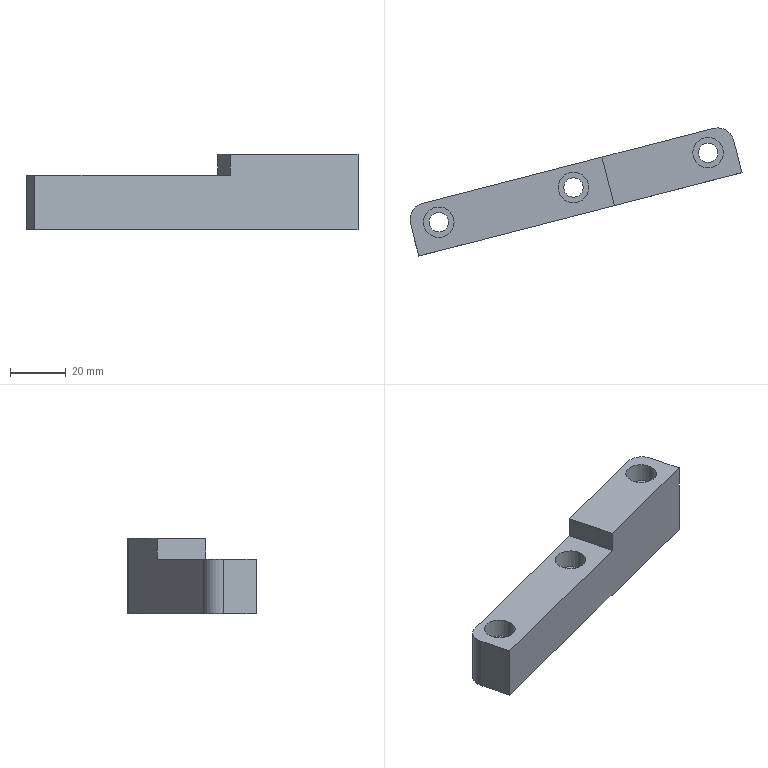Part | STEP file | 车灯-后视镜_id210_x_t | 1 solid | 19 faces | box 119.383 x 46.093 x 27 mm | volume 44427 mm3 | plane 11 | cylinder 8 | commonest cylinder face diameters 7 x3 11 x3 12 x2
STEP:
#1=CARTESIAN_POINT('',(-193.766,-114.635,0.3528));
#2=VERTEX_POINT('',#1);
#3=CARTESIAN_POINT('',(-190.769,-126.254,0.3528));
#4=VERTEX_POINT('',#3);
#5=CARTESIAN_POINT('',(-183.276,-155.303,0.3528));
#6=DIRECTION('',(0.2498,-0.9683,0.));
#7=VECTOR('',#6,1.);
#8=LINE('',#5,#7);
#9=EDGE_CURVE('',#2,#4,#8,.T.);
#10=ORIENTED_EDGE('',*,*,#9,.F.);
#11=CARTESIAN_POINT('',(-193.766,-114.635,-19.147));
#12=VERTEX_POINT('',#11);
#13=CARTESIAN_POINT('',(-193.766,-114.635,-10.327));
#14=DIRECTION('',(0.,0.,-1.));
#15=VECTOR('',#14,1.);
#16=LINE('',#13,#15);
#17=EDGE_CURVE('',#2,#12,#16,.T.);
#18=ORIENTED_EDGE('',*,*,#17,.T.);
#19=CARTESIAN_POINT('',(-190.769,-126.254,-19.147));
#20=VERTEX_POINT('',#19);
#21=CARTESIAN_POINT('',(-183.276,-155.303,-19.147));
#22=DIRECTION('',(0.2498,-0.9683,0.));
#23=VECTOR('',#22,1.);
#24=LINE('',#21,#23);
#25=EDGE_CURVE('',#12,#20,#24,.T.);
#26=ORIENTED_EDGE('',*,*,#25,.T.);
#27=CARTESIAN_POINT('',(-190.769,-126.254,-10.147));
#28=DIRECTION('',(0.,0.,-1.));
#29=VECTOR('',#28,1.);
#30=LINE('',#27,#29);
#31=EDGE_CURVE('',#4,#20,#30,.T.);
#32=ORIENTED_EDGE('',*,*,#31,.F.);
#33=EDGE_LOOP('',(#10,#18,#26,#32));
#34=FACE_OUTER_BOUND('',#33,.T.);
#35=CARTESIAN_POINT('',(-183.276,-155.303,-10.327));
#36=DIRECTION('',(-0.9683,-0.2498,0.));
#37=DIRECTION('',(0.,0.,1.));
#38=AXIS2_PLACEMENT_3D('',#35,#36,#37);
#39=PLANE('',#38);
#40=ADVANCED_FACE('',(#34),#39,.T.);
#41=CARTESIAN_POINT('',(-84.878,-80.352,-19.147));
#42=VERTEX_POINT('',#41);
#43=CARTESIAN_POINT('',(-189.454,-107.326,-19.147));
#44=VERTEX_POINT('',#43);
#45=CARTESIAN_POINT('',(-79.068,-78.853,-19.147));
#46=DIRECTION('',(-0.9683,-0.2498,0.));
#47=VECTOR('',#46,1.);
#48=LINE('',#45,#47);
#49=EDGE_CURVE('',#42,#44,#48,.T.);
#50=ORIENTED_EDGE('',*,*,#49,.T.);
#51=CARTESIAN_POINT('',(-189.454,-107.326,0.3528));
#52=VERTEX_POINT('',#51);
#53=CARTESIAN_POINT('',(-189.454,-107.326,-10.147));
#54=DIRECTION('',(0.,0.,1.));
#55=VECTOR('',#54,1.);
#56=LINE('',#53,#55);
#57=EDGE_CURVE('',#44,#52,#56,.T.);
#58=ORIENTED_EDGE('',*,*,#57,.T.);
#59=CARTESIAN_POINT('',(-124.933,-90.683,0.3528));
#60=VERTEX_POINT('',#59);
#61=CARTESIAN_POINT('',(14.138,-54.811,0.3528));
#62=DIRECTION('',(0.9683,0.2498,0.));
#63=VECTOR('',#62,1.);
#64=LINE('',#61,#63);
#65=EDGE_CURVE('',#52,#60,#64,.T.);
#66=ORIENTED_EDGE('',*,*,#65,.T.);
#67=CARTESIAN_POINT('',(-124.933,-90.683,7.853));
#68=VERTEX_POINT('',#67);
#69=CARTESIAN_POINT('',(-124.933,-90.683,-10.147));
#70=DIRECTION('',(0.,0.,1.));
#71=VECTOR('',#70,1.);
#72=LINE('',#69,#71);
#73=EDGE_CURVE('',#60,#68,#72,.T.);
#74=ORIENTED_EDGE('',*,*,#73,.T.);
#75=CARTESIAN_POINT('',(-84.878,-80.352,7.853));
#76=VERTEX_POINT('',#75);
#77=CARTESIAN_POINT('',(14.138,-54.811,7.853));
#78=DIRECTION('',(0.9683,0.2498,0.));
#79=VECTOR('',#78,1.);
#80=LINE('',#77,#79);
#81=EDGE_CURVE('',#68,#76,#80,.T.);
#82=ORIENTED_EDGE('',*,*,#81,.T.);
#83=CARTESIAN_POINT('',(-84.878,-80.352,-10.147));
#84=DIRECTION('',(0.,0.,-1.));
#85=VECTOR('',#84,1.);
#86=LINE('',#83,#85);
#87=EDGE_CURVE('',#76,#42,#86,.T.);
#88=ORIENTED_EDGE('',*,*,#87,.T.);
#89=EDGE_LOOP('',(#50,#58,#66,#74,#82,#88));
#90=FACE_OUTER_BOUND('',#89,.T.);
#91=CARTESIAN_POINT('',(-127.484,-91.341,-10.147));
#92=DIRECTION('',(-0.2498,0.9683,0.));
#93=DIRECTION('',(0.,0.,1.));
#94=AXIS2_PLACEMENT_3D('',#91,#92,#93);
#95=PLANE('',#94);
#96=ADVANCED_FACE('',(#90),#95,.T.);
#97=CARTESIAN_POINT('',(-74.573,-96.283,-19.147));
#98=VERTEX_POINT('',#97);
#99=CARTESIAN_POINT('',(-74.573,-96.283,-19.147));
#100=DIRECTION('',(-0.9683,-0.2498,0.));
#101=VECTOR('',#100,1.);
#102=LINE('',#99,#101);
#103=EDGE_CURVE('',#98,#20,#102,.T.);
#104=ORIENTED_EDGE('',*,*,#103,.F.);
#105=CARTESIAN_POINT('',(-74.573,-96.283,7.853));
#106=VERTEX_POINT('',#105);
#107=CARTESIAN_POINT('',(-74.573,-96.283,-10.147));
#108=DIRECTION('',(0.,0.,1.));
#109=VECTOR('',#108,1.);
#110=LINE('',#107,#109);
#111=EDGE_CURVE('',#98,#106,#110,.T.);
#112=ORIENTED_EDGE('',*,*,#111,.T.);
#113=CARTESIAN_POINT('',(-120.438,-108.113,7.853));
#114=VERTEX_POINT('',#113);
#115=CARTESIAN_POINT('',(18.634,-72.241,7.853));
#116=DIRECTION('',(0.9683,0.2498,0.));
#117=VECTOR('',#116,1.);
#118=LINE('',#115,#117);
#119=EDGE_CURVE('',#114,#106,#118,.T.);
#120=ORIENTED_EDGE('',*,*,#119,.F.);
#121=CARTESIAN_POINT('',(-120.438,-108.113,0.3528));
#122=VERTEX_POINT('',#121);
#123=CARTESIAN_POINT('',(-120.438,-108.113,-10.147));
#124=DIRECTION('',(0.,0.,1.));
#125=VECTOR('',#124,1.);
#126=LINE('',#123,#125);
#127=EDGE_CURVE('',#122,#114,#126,.T.);
#128=ORIENTED_EDGE('',*,*,#127,.F.);
#129=CARTESIAN_POINT('',(18.634,-72.241,0.3528));
#130=DIRECTION('',(0.9683,0.2498,0.));
#131=VECTOR('',#130,1.);
#132=LINE('',#129,#131);
#133=EDGE_CURVE('',#4,#122,#132,.T.);
#134=ORIENTED_EDGE('',*,*,#133,.F.);
#135=ORIENTED_EDGE('',*,*,#31,.T.);
#136=EDGE_LOOP('',(#104,#112,#120,#128,#134,#135));
#137=FACE_OUTER_BOUND('',#136,.T.);
#138=CARTESIAN_POINT('',(-122.988,-108.771,-10.147));
#139=DIRECTION('',(-0.2498,0.9683,0.));
#140=DIRECTION('',(0.,0.,1.));
#141=AXIS2_PLACEMENT_3D('',#138,#139,#140);
#142=PLANE('',#141);
#143=ADVANCED_FACE('',(#137),#142,.F.);
#144=CARTESIAN_POINT('',(-129.668,-101.585,0.3528));
#145=VERTEX_POINT('',#144);
#146=CARTESIAN_POINT('',(-135.168,-101.585,0.3528));
#147=DIRECTION('',(0.,0.,-1.));
#148=DIRECTION('',(1.,0.,0.));
#149=AXIS2_PLACEMENT_3D('',#146,#147,#148);
#150=CIRCLE('',#149,5.5);
#151=EDGE_CURVE('',#145,#145,#150,.T.);
#152=ORIENTED_EDGE('',*,*,#151,.T.);
#153=EDGE_LOOP('',(#152));
#154=FACE_BOUND('',#153,.T.);
#155=CARTESIAN_POINT('',(-178.083,-114.073,0.3528));
#156=VERTEX_POINT('',#155);
#157=CARTESIAN_POINT('',(-183.583,-114.073,0.3528));
#158=DIRECTION('',(0.,0.,-1.));
#159=DIRECTION('',(1.,0.,0.));
#160=AXIS2_PLACEMENT_3D('',#157,#158,#159);
#161=CIRCLE('',#160,5.5);
#162=EDGE_CURVE('',#156,#156,#161,.T.);
#163=ORIENTED_EDGE('',*,*,#162,.T.);
#164=EDGE_LOOP('',(#163));
#165=FACE_BOUND('',#164,.T.);
#166=ORIENTED_EDGE('',*,*,#65,.F.);
#167=CARTESIAN_POINT('',(-187.956,-113.136,0.3528));
#168=DIRECTION('',(0.,0.,1.));
#169=DIRECTION('',(1.,0.,0.));
#170=AXIS2_PLACEMENT_3D('',#167,#168,#169);
#171=CIRCLE('',#170,6.);
#172=EDGE_CURVE('',#52,#2,#171,.T.);
#173=ORIENTED_EDGE('',*,*,#172,.T.);
#174=ORIENTED_EDGE('',*,*,#9,.T.);
#175=ORIENTED_EDGE('',*,*,#133,.T.);
#176=CARTESIAN_POINT('',(-139.071,-35.872,0.3528));
#177=DIRECTION('',(-0.2498,0.9683,0.));
#178=VECTOR('',#177,1.);
#179=LINE('',#176,#178);
#180=EDGE_CURVE('',#122,#60,#179,.T.);
#181=ORIENTED_EDGE('',*,*,#180,.T.);
#182=EDGE_LOOP('',(#166,#173,#174,#175,#181));
#183=FACE_BOUND('',#182,.T.);
#184=CARTESIAN_POINT('',(0.,0.,0.3528));
#185=DIRECTION('',(0.,0.,1.));
#186=DIRECTION('',(1.,0.,0.));
#187=AXIS2_PLACEMENT_3D('',#184,#185,#186);
#188=PLANE('',#187);
#189=ADVANCED_FACE('',(#154,#165,#183),#188,.T.);
#190=CARTESIAN_POINT('',(-90.252,-89.097,-19.147));
#191=VERTEX_POINT('',#190);
#192=CARTESIAN_POINT('',(-86.752,-89.097,-19.147));
#193=DIRECTION('',(0.,0.,1.));
#194=DIRECTION('',(-1.,0.,0.));
#195=AXIS2_PLACEMENT_3D('',#192,#193,#194);
#196=CIRCLE('',#195,3.5);
#197=EDGE_CURVE('',#191,#191,#196,.T.);
#198=ORIENTED_EDGE('',*,*,#197,.T.);
#199=EDGE_LOOP('',(#198));
#200=FACE_BOUND('',#199,.T.);
#201=CARTESIAN_POINT('',(-138.668,-101.585,-19.147));
#202=VERTEX_POINT('',#201);
#203=CARTESIAN_POINT('',(-135.168,-101.585,-19.147));
#204=DIRECTION('',(0.,0.,1.));
#205=DIRECTION('',(-1.,0.,0.));
#206=AXIS2_PLACEMENT_3D('',#203,#204,#205);
#207=CIRCLE('',#206,3.5);
#208=EDGE_CURVE('',#202,#202,#207,.T.);
#209=ORIENTED_EDGE('',*,*,#208,.T.);
#210=EDGE_LOOP('',(#209));
#211=FACE_BOUND('',#210,.T.);
#212=CARTESIAN_POINT('',(-187.083,-114.073,-19.147));
#213=VERTEX_POINT('',#212);
#214=CARTESIAN_POINT('',(-183.583,-114.073,-19.147));
#215=DIRECTION('',(0.,0.,1.));
#216=DIRECTION('',(-1.,0.,0.));
#217=AXIS2_PLACEMENT_3D('',#214,#215,#216);
#218=CIRCLE('',#217,3.5);
#219=EDGE_CURVE('',#213,#213,#218,.T.);
#220=ORIENTED_EDGE('',*,*,#219,.T.);
#221=EDGE_LOOP('',(#220));
#222=FACE_BOUND('',#221,.T.);
#223=ORIENTED_EDGE('',*,*,#25,.F.);
#224=CARTESIAN_POINT('',(-187.956,-113.136,-19.147));
#225=DIRECTION('',(0.,0.,-1.));
#226=DIRECTION('',(1.,0.,0.));
#227=AXIS2_PLACEMENT_3D('',#224,#225,#226);
#228=CIRCLE('',#227,6.);
#229=EDGE_CURVE('',#12,#44,#228,.T.);
#230=ORIENTED_EDGE('',*,*,#229,.T.);
#231=ORIENTED_EDGE('',*,*,#49,.F.);
#232=CARTESIAN_POINT('',(-77.57,-84.663,-19.147));
#233=VERTEX_POINT('',#232);
#234=CARTESIAN_POINT('',(-83.38,-86.162,-19.147));
#235=DIRECTION('',(0.,0.,-1.));
#236=DIRECTION('',(1.,0.,0.));
#237=AXIS2_PLACEMENT_3D('',#234,#235,#236);
#238=CIRCLE('',#237,6.);
#239=EDGE_CURVE('',#42,#233,#238,.T.);
#240=ORIENTED_EDGE('',*,*,#239,.T.);
#241=CARTESIAN_POINT('',(-79.068,-78.853,-19.147));
#242=DIRECTION('',(0.2498,-0.9683,0.));
#243=VECTOR('',#242,1.);
#244=LINE('',#241,#243);
#245=EDGE_CURVE('',#233,#98,#244,.T.);
#246=ORIENTED_EDGE('',*,*,#245,.T.);
#247=ORIENTED_EDGE('',*,*,#103,.T.);
#248=EDGE_LOOP('',(#223,#230,#231,#240,#246,#247));
#249=FACE_BOUND('',#248,.T.);
#250=CARTESIAN_POINT('',(-79.068,-78.853,-19.147));
#251=DIRECTION('',(0.,0.,1.));
#252=DIRECTION('',(1.,0.,0.));
#253=AXIS2_PLACEMENT_3D('',#250,#251,#252);
#254=PLANE('',#253);
#255=ADVANCED_FACE('',(#200,#211,#222,#249),#254,.F.);
#256=ORIENTED_EDGE('',*,*,#180,.F.);
#257=ORIENTED_EDGE('',*,*,#127,.T.);
#258=CARTESIAN_POINT('',(-139.071,-35.872,7.853));
#259=DIRECTION('',(-0.2498,0.9683,0.));
#260=VECTOR('',#259,1.);
#261=LINE('',#258,#260);
#262=EDGE_CURVE('',#114,#68,#261,.T.);
#263=ORIENTED_EDGE('',*,*,#262,.T.);
#264=ORIENTED_EDGE('',*,*,#73,.F.);
#265=EDGE_LOOP('',(#256,#257,#263,#264));
#266=FACE_OUTER_BOUND('',#265,.T.);
#267=CARTESIAN_POINT('',(-122.685,-99.398,0.3528));
#268=DIRECTION('',(-0.9683,-0.2498,0.));
#269=DIRECTION('',(0.2498,-0.9683,0.));
#270=AXIS2_PLACEMENT_3D('',#267,#268,#269);
#271=PLANE('',#270);
#272=ADVANCED_FACE('',(#266),#271,.T.);
#273=CARTESIAN_POINT('',(-81.252,-89.097,7.853));
#274=VERTEX_POINT('',#273);
#275=CARTESIAN_POINT('',(-86.752,-89.097,7.853));
#276=DIRECTION('',(0.,0.,-1.));
#277=DIRECTION('',(1.,0.,0.));
#278=AXIS2_PLACEMENT_3D('',#275,#276,#277);
#279=CIRCLE('',#278,5.5);
#280=EDGE_CURVE('',#274,#274,#279,.T.);
#281=ORIENTED_EDGE('',*,*,#280,.T.);
#282=EDGE_LOOP('',(#281));
#283=FACE_BOUND('',#282,.T.);
#284=CARTESIAN_POINT('',(-77.57,-84.663,7.853));
#285=VERTEX_POINT('',#284);
#286=CARTESIAN_POINT('',(-93.206,-24.042,7.853));
#287=DIRECTION('',(0.2498,-0.9683,0.));
#288=VECTOR('',#287,1.);
#289=LINE('',#286,#288);
#290=EDGE_CURVE('',#285,#106,#289,.T.);
#291=ORIENTED_EDGE('',*,*,#290,.F.);
#292=CARTESIAN_POINT('',(-83.38,-86.162,7.853));
#293=DIRECTION('',(0.,0.,1.));
#294=DIRECTION('',(1.,0.,0.));
#295=AXIS2_PLACEMENT_3D('',#292,#293,#294);
#296=CIRCLE('',#295,6.);
#297=EDGE_CURVE('',#285,#76,#296,.T.);
#298=ORIENTED_EDGE('',*,*,#297,.T.);
#299=ORIENTED_EDGE('',*,*,#81,.F.);
#300=ORIENTED_EDGE('',*,*,#262,.F.);
#301=ORIENTED_EDGE('',*,*,#119,.T.);
#302=EDGE_LOOP('',(#291,#298,#299,#300,#301));
#303=FACE_BOUND('',#302,.T.);
#304=CARTESIAN_POINT('',(0.,0.,7.853));
#305=DIRECTION('',(0.,0.,1.));
#306=DIRECTION('',(1.,0.,0.));
#307=AXIS2_PLACEMENT_3D('',#304,#305,#306);
#308=PLANE('',#307);
#309=ADVANCED_FACE('',(#283,#303),#308,.T.);
#310=ORIENTED_EDGE('',*,*,#245,.F.);
#311=CARTESIAN_POINT('',(-77.57,-84.663,-10.147));
#312=DIRECTION('',(0.,0.,1.));
#313=VECTOR('',#312,1.);
#314=LINE('',#311,#313);
#315=EDGE_CURVE('',#233,#285,#314,.T.);
#316=ORIENTED_EDGE('',*,*,#315,.T.);
#317=ORIENTED_EDGE('',*,*,#290,.T.);
#318=ORIENTED_EDGE('',*,*,#111,.F.);
#319=EDGE_LOOP('',(#310,#316,#317,#318));
#320=FACE_OUTER_BOUND('',#319,.T.);
#321=CARTESIAN_POINT('',(-79.068,-78.853,-10.147));
#322=DIRECTION('',(0.9683,0.2498,0.));
#323=DIRECTION('',(-0.2498,0.9683,0.));
#324=AXIS2_PLACEMENT_3D('',#321,#322,#323);
#325=PLANE('',#324);
#326=ADVANCED_FACE('',(#320),#325,.T.);
#327=ORIENTED_EDGE('',*,*,#172,.F.);
#328=ORIENTED_EDGE('',*,*,#57,.F.);
#329=ORIENTED_EDGE('',*,*,#229,.F.);
#330=ORIENTED_EDGE('',*,*,#17,.F.);
#331=EDGE_LOOP('',(#327,#328,#329,#330));
#332=FACE_OUTER_BOUND('',#331,.T.);
#333=CARTESIAN_POINT('',(-187.956,-113.136,-10.327));
#334=DIRECTION('',(0.,0.,-1.));
#335=DIRECTION('',(-1.,0.,0.));
#336=AXIS2_PLACEMENT_3D('',#333,#334,#335);
#337=CYLINDRICAL_SURFACE('',#336,6.);
#338=ADVANCED_FACE('',(#332),#337,.T.);
#339=ORIENTED_EDGE('',*,*,#239,.F.);
#340=ORIENTED_EDGE('',*,*,#87,.F.);
#341=ORIENTED_EDGE('',*,*,#297,.F.);
#342=ORIENTED_EDGE('',*,*,#315,.F.);
#343=EDGE_LOOP('',(#339,#340,#341,#342));
#344=FACE_OUTER_BOUND('',#343,.T.);
#345=CARTESIAN_POINT('',(-83.38,-86.162,-10.147));
#346=DIRECTION('',(0.,0.,1.));
#347=DIRECTION('',(1.,0.,0.));
#348=AXIS2_PLACEMENT_3D('',#345,#346,#347);
#349=CYLINDRICAL_SURFACE('',#348,6.);
#350=ADVANCED_FACE('',(#344),#349,.T.);
#351=CARTESIAN_POINT('',(-187.083,-114.073,-6.647));
#352=VERTEX_POINT('',#351);
#353=CARTESIAN_POINT('',(-183.583,-114.073,-6.647));
#354=DIRECTION('',(0.,0.,1.));
#355=DIRECTION('',(-1.,0.,0.));
#356=AXIS2_PLACEMENT_3D('',#353,#354,#355);
#357=CIRCLE('',#356,3.5);
#358=EDGE_CURVE('',#352,#352,#357,.T.);
#359=ORIENTED_EDGE('',*,*,#358,.T.);
#360=EDGE_LOOP('',(#359));
#361=FACE_BOUND('',#360,.T.);
#362=ORIENTED_EDGE('',*,*,#219,.F.);
#363=EDGE_LOOP('',(#362));
#364=FACE_BOUND('',#363,.T.);
#365=CARTESIAN_POINT('',(-183.583,-114.073,-19.147));
#366=DIRECTION('',(0.,0.,1.));
#367=DIRECTION('',(-1.,0.,0.));
#368=AXIS2_PLACEMENT_3D('',#365,#366,#367);
#369=CYLINDRICAL_SURFACE('',#368,3.5);
#370=ADVANCED_FACE('',(#361,#364),#369,.F.);
#371=ORIENTED_EDGE('',*,*,#358,.F.);
#372=EDGE_LOOP('',(#371));
#373=FACE_BOUND('',#372,.T.);
#374=CARTESIAN_POINT('',(-189.083,-114.073,-6.647));
#375=VERTEX_POINT('',#374);
#376=CARTESIAN_POINT('',(-183.583,-114.073,-6.647));
#377=DIRECTION('',(0.,0.,1.));
#378=DIRECTION('',(-1.,0.,0.));
#379=AXIS2_PLACEMENT_3D('',#376,#377,#378);
#380=CIRCLE('',#379,5.5);
#381=EDGE_CURVE('',#375,#375,#380,.T.);
#382=ORIENTED_EDGE('',*,*,#381,.T.);
#383=EDGE_LOOP('',(#382));
#384=FACE_BOUND('',#383,.T.);
#385=CARTESIAN_POINT('',(-183.583,-114.073,-6.647));
#386=DIRECTION('',(0.,0.,-1.));
#387=DIRECTION('',(1.,0.,0.));
#388=AXIS2_PLACEMENT_3D('',#385,#386,#387);
#389=PLANE('',#388);
#390=ADVANCED_FACE('',(#373,#384),#389,.F.);
#391=ORIENTED_EDGE('',*,*,#381,.F.);
#392=EDGE_LOOP('',(#391));
#393=FACE_BOUND('',#392,.T.);
#394=ORIENTED_EDGE('',*,*,#162,.F.);
#395=EDGE_LOOP('',(#394));
#396=FACE_BOUND('',#395,.T.);
#397=CARTESIAN_POINT('',(-183.583,-114.073,0.3528));
#398=DIRECTION('',(0.,0.,-1.));
#399=DIRECTION('',(1.,0.,0.));
#400=AXIS2_PLACEMENT_3D('',#397,#398,#399);
#401=CYLINDRICAL_SURFACE('',#400,5.5);
#402=ADVANCED_FACE('',(#393,#396),#401,.F.);
#403=CARTESIAN_POINT('',(-138.668,-101.585,-6.647));
#404=VERTEX_POINT('',#403);
#405=CARTESIAN_POINT('',(-135.168,-101.585,-6.647));
#406=DIRECTION('',(0.,0.,1.));
#407=DIRECTION('',(-1.,0.,0.));
#408=AXIS2_PLACEMENT_3D('',#405,#406,#407);
#409=CIRCLE('',#408,3.5);
#410=EDGE_CURVE('',#404,#404,#409,.T.);
#411=ORIENTED_EDGE('',*,*,#410,.T.);
#412=EDGE_LOOP('',(#411));
#413=FACE_BOUND('',#412,.T.);
#414=ORIENTED_EDGE('',*,*,#208,.F.);
#415=EDGE_LOOP('',(#414));
#416=FACE_BOUND('',#415,.T.);
#417=CARTESIAN_POINT('',(-135.168,-101.585,-19.147));
#418=DIRECTION('',(0.,0.,1.));
#419=DIRECTION('',(-1.,0.,0.));
#420=AXIS2_PLACEMENT_3D('',#417,#418,#419);
#421=CYLINDRICAL_SURFACE('',#420,3.5);
#422=ADVANCED_FACE('',(#413,#416),#421,.F.);
#423=ORIENTED_EDGE('',*,*,#410,.F.);
#424=EDGE_LOOP('',(#423));
#425=FACE_BOUND('',#424,.T.);
#426=CARTESIAN_POINT('',(-140.668,-101.585,-6.647));
#427=VERTEX_POINT('',#426);
#428=CARTESIAN_POINT('',(-135.168,-101.585,-6.647));
#429=DIRECTION('',(0.,0.,1.));
#430=DIRECTION('',(-1.,0.,0.));
#431=AXIS2_PLACEMENT_3D('',#428,#429,#430);
#432=CIRCLE('',#431,5.5);
#433=EDGE_CURVE('',#427,#427,#432,.T.);
#434=ORIENTED_EDGE('',*,*,#433,.T.);
#435=EDGE_LOOP('',(#434));
#436=FACE_BOUND('',#435,.T.);
#437=CARTESIAN_POINT('',(-135.168,-101.585,-6.647));
#438=DIRECTION('',(0.,0.,-1.));
#439=DIRECTION('',(1.,0.,0.));
#440=AXIS2_PLACEMENT_3D('',#437,#438,#439);
#441=PLANE('',#440);
#442=ADVANCED_FACE('',(#425,#436),#441,.F.);
#443=ORIENTED_EDGE('',*,*,#433,.F.);
#444=EDGE_LOOP('',(#443));
#445=FACE_BOUND('',#444,.T.);
#446=ORIENTED_EDGE('',*,*,#151,.F.);
#447=EDGE_LOOP('',(#446));
#448=FACE_BOUND('',#447,.T.);
#449=CARTESIAN_POINT('',(-135.168,-101.585,0.3528));
#450=DIRECTION('',(0.,0.,-1.));
#451=DIRECTION('',(1.,0.,0.));
#452=AXIS2_PLACEMENT_3D('',#449,#450,#451);
#453=CYLINDRICAL_SURFACE('',#452,5.5);
#454=ADVANCED_FACE('',(#445,#448),#453,.F.);
#455=CARTESIAN_POINT('',(-90.252,-89.097,0.8528));
#456=VERTEX_POINT('',#455);
#457=CARTESIAN_POINT('',(-86.752,-89.097,0.8528));
#458=DIRECTION('',(0.,0.,1.));
#459=DIRECTION('',(-1.,0.,0.));
#460=AXIS2_PLACEMENT_3D('',#457,#458,#459);
#461=CIRCLE('',#460,3.5);
#462=EDGE_CURVE('',#456,#456,#461,.T.);
#463=ORIENTED_EDGE('',*,*,#462,.T.);
#464=EDGE_LOOP('',(#463));
#465=FACE_BOUND('',#464,.T.);
#466=ORIENTED_EDGE('',*,*,#197,.F.);
#467=EDGE_LOOP('',(#466));
#468=FACE_BOUND('',#467,.T.);
#469=CARTESIAN_POINT('',(-86.752,-89.097,-19.147));
#470=DIRECTION('',(0.,0.,1.));
#471=DIRECTION('',(-1.,0.,0.));
#472=AXIS2_PLACEMENT_3D('',#469,#470,#471);
#473=CYLINDRICAL_SURFACE('',#472,3.5);
#474=ADVANCED_FACE('',(#465,#468),#473,.F.);
#475=ORIENTED_EDGE('',*,*,#462,.F.);
#476=EDGE_LOOP('',(#475));
#477=FACE_BOUND('',#476,.T.);
#478=CARTESIAN_POINT('',(-92.252,-89.097,0.8528));
#479=VERTEX_POINT('',#478);
#480=CARTESIAN_POINT('',(-86.752,-89.097,0.8528));
#481=DIRECTION('',(0.,0.,1.));
#482=DIRECTION('',(-1.,0.,0.));
#483=AXIS2_PLACEMENT_3D('',#480,#481,#482);
#484=CIRCLE('',#483,5.5);
#485=EDGE_CURVE('',#479,#479,#484,.T.);
#486=ORIENTED_EDGE('',*,*,#485,.T.);
#487=EDGE_LOOP('',(#486));
#488=FACE_BOUND('',#487,.T.);
#489=CARTESIAN_POINT('',(-86.752,-89.097,0.8528));
#490=DIRECTION('',(0.,0.,-1.));
#491=DIRECTION('',(1.,0.,0.));
#492=AXIS2_PLACEMENT_3D('',#489,#490,#491);
#493=PLANE('',#492);
#494=ADVANCED_FACE('',(#477,#488),#493,.F.);
#495=ORIENTED_EDGE('',*,*,#485,.F.);
#496=EDGE_LOOP('',(#495));
#497=FACE_BOUND('',#496,.T.);
#498=ORIENTED_EDGE('',*,*,#280,.F.);
#499=EDGE_LOOP('',(#498));
#500=FACE_BOUND('',#499,.T.);
#501=CARTESIAN_POINT('',(-86.752,-89.097,7.853));
#502=DIRECTION('',(0.,0.,-1.));
#503=DIRECTION('',(1.,0.,0.));
#504=AXIS2_PLACEMENT_3D('',#501,#502,#503);
#505=CYLINDRICAL_SURFACE('',#504,5.5);
#506=ADVANCED_FACE('',(#497,#500),#505,.F.);
#507=CLOSED_SHELL('',(#40,#96,#143,#189,#255,#272,#309,#326,#338,#350,#370,#390,#402,#422,#442,#454,#474,#494,#506));
#508=MANIFOLD_SOLID_BREP('',#507);
#509=(LENGTH_UNIT()NAMED_UNIT(*)SI_UNIT(.MILLI.,.METRE.));
#510=UNCERTAINTY_MEASURE_WITH_UNIT(LENGTH_MEASURE(0.00002),#509,'','');
#511=(NAMED_UNIT(*)PLANE_ANGLE_UNIT()SI_UNIT($,.RADIAN.));
#512=PLANE_ANGLE_MEASURE_WITH_UNIT(PLANE_ANGLE_MEASURE(0.01745),#511);
#513=DIMENSIONAL_EXPONENTS(0.,0.,0.,0.,0.,0.,0.);
#514=(CONVERSION_BASED_UNIT('DEGREE',#512)NAMED_UNIT(#513)PLANE_ANGLE_UNIT());
#515=(NAMED_UNIT(*)SI_UNIT($,.STERADIAN.)SOLID_ANGLE_UNIT());
#516=(GEOMETRIC_REPRESENTATION_CONTEXT(3)GLOBAL_UNCERTAINTY_ASSIGNED_CONTEXT((#510))GLOBAL_UNIT_ASSIGNED_CONTEXT((#509,#514,#515))REPRESENTATION_CONTEXT('',''));
#517=ADVANCED_BREP_SHAPE_REPRESENTATION('',(#508),#516);